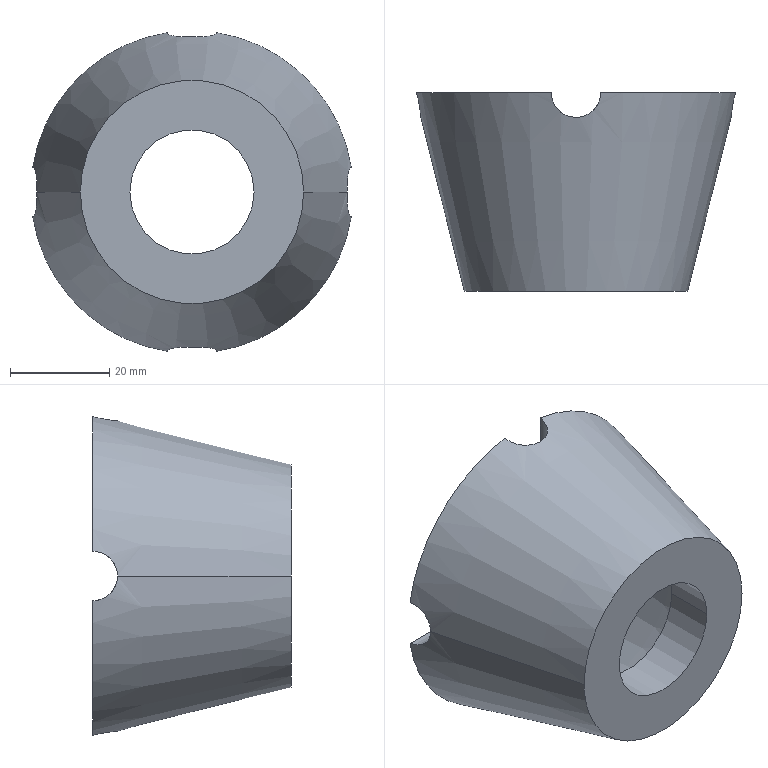Part | SolidWorks | features ICE 2, CirPattern 1, Revolution 1 | 1 solid | 16 faces | box 64.226 x 40 x 64.226 mm | volume 43850 mm3 | cylinder 6 | plane 6 | cone 4 | commonest cylinder face diameters 10 x4 25 x2
STEP:
#1=CARTESIAN_POINT('',(12.5,-20.,0.));
#2=VERTEX_POINT('',#1);
#3=CARTESIAN_POINT('',(-12.5,-20.,0.));
#4=VERTEX_POINT('',#3);
#5=CARTESIAN_POINT('',(0.,-20.,0.));
#6=DIRECTION('',(0.,1.,0.));
#7=DIRECTION('',(-1.,0.,0.));
#8=AXIS2_PLACEMENT_3D('',#5,#6,#7);
#9=CIRCLE('',#8,12.5);
#10=EDGE_CURVE('',#2,#4,#9,.T.);
#11=ORIENTED_EDGE('',*,*,#10,.F.);
#12=CARTESIAN_POINT('',(12.5,-10.,0.));
#13=VERTEX_POINT('',#12);
#14=CARTESIAN_POINT('',(12.5,-20.,0.));
#15=DIRECTION('',(0.,1.,0.));
#16=VECTOR('',#15,1000.);
#17=LINE('',#14,#16);
#18=EDGE_CURVE('',#2,#13,#17,.T.);
#19=ORIENTED_EDGE('',*,*,#18,.T.);
#20=CARTESIAN_POINT('',(-12.5,-10.,0.));
#21=VERTEX_POINT('',#20);
#22=CARTESIAN_POINT('',(0.,-10.,0.));
#23=DIRECTION('',(0.,1.,0.));
#24=DIRECTION('',(-1.,0.,0.));
#25=AXIS2_PLACEMENT_3D('',#22,#23,#24);
#26=CIRCLE('',#25,12.5);
#27=EDGE_CURVE('',#13,#21,#26,.T.);
#28=ORIENTED_EDGE('',*,*,#27,.T.);
#29=CARTESIAN_POINT('',(-12.5,-20.,0.));
#30=DIRECTION('',(0.,1.,0.));
#31=VECTOR('',#30,1000.);
#32=LINE('',#29,#31);
#33=EDGE_CURVE('',#4,#21,#32,.T.);
#34=ORIENTED_EDGE('',*,*,#33,.F.);
#35=EDGE_LOOP('',(#11,#19,#28,#34));
#36=FACE_OUTER_BOUND('',#35,.T.);
#37=CARTESIAN_POINT('',(0.,-20.,0.));
#38=DIRECTION('',(0.,1.,0.));
#39=DIRECTION('',(-1.,0.,0.));
#40=AXIS2_PLACEMENT_3D('',#37,#38,#39);
#41=CYLINDRICAL_SURFACE('',#40,12.5);
#42=ADVANCED_FACE('',(#36),#41,.F.);
#43=CARTESIAN_POINT('',(-22.5,-20.,0.));
#44=VERTEX_POINT('',#43);
#45=CARTESIAN_POINT('',(22.5,-20.,0.));
#46=VERTEX_POINT('',#45);
#47=CARTESIAN_POINT('',(0.,-20.,0.));
#48=DIRECTION('',(0.,1.,0.));
#49=DIRECTION('',(-1.,0.,0.));
#50=AXIS2_PLACEMENT_3D('',#47,#48,#49);
#51=CIRCLE('',#50,22.5);
#52=EDGE_CURVE('',#44,#46,#51,.T.);
#53=ORIENTED_EDGE('',*,*,#52,.T.);
#54=CARTESIAN_POINT('',(31.25,15.,0.));
#55=VERTEX_POINT('',#54);
#56=CARTESIAN_POINT('',(22.5,-20.,0.));
#57=DIRECTION('',(0.2425,0.9701,0.));
#58=VECTOR('',#57,1000.);
#59=LINE('',#56,#58);
#60=EDGE_CURVE('',#46,#55,#59,.T.);
#61=ORIENTED_EDGE('',*,*,#60,.T.);
#62=CARTESIAN_POINT('',(32.113,20.,5.));
#63=VERTEX_POINT('',#62);
#64=CARTESIAN_POINT('',(31.25,15.,0.));
#65=CARTESIAN_POINT('',(31.25,15.,0.3288));
#66=CARTESIAN_POINT('',(31.253,15.033,0.6628));
#67=CARTESIAN_POINT('',(31.265,15.163,1.309));
#68=CARTESIAN_POINT('',(31.274,15.259,1.623));
#69=CARTESIAN_POINT('',(31.294,15.45,2.08));
#70=CARTESIAN_POINT('',(31.301,15.522,2.23));
#71=CARTESIAN_POINT('',(31.319,15.679,2.521));
#72=CARTESIAN_POINT('',(31.328,15.764,2.662));
#73=CARTESIAN_POINT('',(31.361,16.039,3.069));
#74=CARTESIAN_POINT('',(31.388,16.249,3.322));
#75=CARTESIAN_POINT('',(31.453,16.72,3.788));
#76=CARTESIAN_POINT('',(31.492,16.974,3.994));
#77=CARTESIAN_POINT('',(31.581,17.517,4.352));
#78=CARTESIAN_POINT('',(31.633,17.81,4.507));
#79=CARTESIAN_POINT('',(31.749,18.412,4.752));
#80=CARTESIAN_POINT('',(31.813,18.72,4.844));
#81=CARTESIAN_POINT('',(31.954,19.353,4.968));
#82=CARTESIAN_POINT('',(32.031,19.677,5.));
#83=CARTESIAN_POINT('',(32.113,20.,5.));
#84=B_SPLINE_CURVE_WITH_KNOTS('',3,(#64,#65,#66,#67,#68,#69,#70,#71,#72,#73,#74,#75,#76,#77,#78,#79,#80,#81,#82,#83),.UNSPECIFIED.,.F.,.F.,(4,2,2,2,2,2,2,2,2,4),(0.007888,0.008873,0.009858,0.01035,0.01084,0.01183,0.01281,0.0138,0.01478,0.01577),.UNSPECIFIED.);
#85=EDGE_CURVE('',#55,#63,#84,.T.);
#86=ORIENTED_EDGE('',*,*,#85,.T.);
#87=CARTESIAN_POINT('',(5.,20.,32.113));
#88=VERTEX_POINT('',#87);
#89=CARTESIAN_POINT('',(0.,20.,0.));
#90=DIRECTION('',(0.,1.,0.));
#91=DIRECTION('',(-1.,0.,0.));
#92=AXIS2_PLACEMENT_3D('',#89,#90,#91);
#93=CIRCLE('',#92,32.5);
#94=EDGE_CURVE('',#88,#63,#93,.T.);
#95=ORIENTED_EDGE('',*,*,#94,.F.);
#96=CARTESIAN_POINT('',(-5.,20.,32.113));
#97=VERTEX_POINT('',#96);
#98=CARTESIAN_POINT('',(5.,20.,32.113));
#99=CARTESIAN_POINT('',(5.,19.677,32.031));
#100=CARTESIAN_POINT('',(4.969,19.358,31.956));
#101=CARTESIAN_POINT('',(4.877,18.886,31.85));
#102=CARTESIAN_POINT('',(4.838,18.729,31.816));
#103=CARTESIAN_POINT('',(4.746,18.418,31.752));
#104=CARTESIAN_POINT('',(4.691,18.263,31.721));
#105=CARTESIAN_POINT('',(4.507,17.811,31.633));
#106=CARTESIAN_POINT('',(4.356,17.524,31.582));
#107=CARTESIAN_POINT('',(3.997,16.979,31.492));
#108=CARTESIAN_POINT('',(3.787,16.719,31.453));
#109=CARTESIAN_POINT('',(3.327,16.253,31.388));
#110=CARTESIAN_POINT('',(3.075,16.044,31.362));
#111=CARTESIAN_POINT('',(2.665,15.766,31.329));
#112=CARTESIAN_POINT('',(2.522,15.679,31.319));
#113=CARTESIAN_POINT('',(2.231,15.523,31.302));
#114=CARTESIAN_POINT('',(2.083,15.452,31.294));
#115=CARTESIAN_POINT('',(1.629,15.261,31.274));
#116=CARTESIAN_POINT('',(1.312,15.164,31.265));
#117=CARTESIAN_POINT('',(0.6608,15.033,31.253));
#118=CARTESIAN_POINT('',(0.3335,15.,31.25));
#119=CARTESIAN_POINT('',(-0.3245,15.,31.25));
#120=CARTESIAN_POINT('',(-0.6586,15.033,31.253));
#121=CARTESIAN_POINT('',(-1.305,15.162,31.265));
#122=CARTESIAN_POINT('',(-1.619,15.258,31.274));
#123=CARTESIAN_POINT('',(-2.077,15.449,31.294));
#124=CARTESIAN_POINT('',(-2.228,15.521,31.301));
#125=CARTESIAN_POINT('',(-2.519,15.677,31.319));
#126=CARTESIAN_POINT('',(-2.659,15.763,31.328));
#127=CARTESIAN_POINT('',(-3.067,16.038,31.361));
#128=CARTESIAN_POINT('',(-3.32,16.247,31.387));
#129=CARTESIAN_POINT('',(-3.787,16.718,31.453));
#130=CARTESIAN_POINT('',(-3.992,16.972,31.491));
#131=CARTESIAN_POINT('',(-4.351,17.516,31.581));
#132=CARTESIAN_POINT('',(-4.506,17.809,31.633));
#133=CARTESIAN_POINT('',(-4.752,18.411,31.749));
#134=CARTESIAN_POINT('',(-4.844,18.72,31.813));
#135=CARTESIAN_POINT('',(-4.968,19.353,31.954));
#136=CARTESIAN_POINT('',(-5.,19.677,32.031));
#137=CARTESIAN_POINT('',(-5.,20.,32.113));
#138=B_SPLINE_CURVE_WITH_KNOTS('',3,(#98,#99,#100,#101,#102,#103,#104,#105,#106,#107,#108,#109,#110,#111,#112,#113,#114,#115,#116,#117,#118,#119,#120,#121,#122,#123,#124,#125,#126,#127,#128,#129,#130,#131,#132,#133,#134,#135,#136,#137),.UNSPECIFIED.,.F.,.F.,(4,2,2,2,2,2,2,2,2,2,2,2,2,2,2,2,2,2,2,4),(0.000000203,0.0009857,0.001478,0.001971,0.002957,0.003942,0.004927,0.00542,0.005913,0.006898,0.007884,0.008869,0.009855,0.01035,0.01084,0.01183,0.01281,0.0138,0.01478,0.01577),.UNSPECIFIED.);
#139=EDGE_CURVE('',#88,#97,#138,.T.);
#140=ORIENTED_EDGE('',*,*,#139,.T.);
#141=CARTESIAN_POINT('',(-32.113,20.,5.));
#142=VERTEX_POINT('',#141);
#143=CARTESIAN_POINT('',(0.,20.,0.));
#144=DIRECTION('',(0.,1.,0.));
#145=DIRECTION('',(-1.,0.,0.));
#146=AXIS2_PLACEMENT_3D('',#143,#144,#145);
#147=CIRCLE('',#146,32.5);
#148=EDGE_CURVE('',#142,#97,#147,.T.);
#149=ORIENTED_EDGE('',*,*,#148,.F.);
#150=CARTESIAN_POINT('',(-31.25,15.,0.));
#151=VERTEX_POINT('',#150);
#152=CARTESIAN_POINT('',(-32.113,20.,5.));
#153=CARTESIAN_POINT('',(-32.031,19.677,5.));
#154=CARTESIAN_POINT('',(-31.955,19.358,4.969));
#155=CARTESIAN_POINT('',(-31.85,18.885,4.877));
#156=CARTESIAN_POINT('',(-31.816,18.728,4.838));
#157=CARTESIAN_POINT('',(-31.752,18.417,4.746));
#158=CARTESIAN_POINT('',(-31.721,18.262,4.691));
#159=CARTESIAN_POINT('',(-31.633,17.81,4.506));
#160=CARTESIAN_POINT('',(-31.582,17.522,4.355));
#161=CARTESIAN_POINT('',(-31.492,16.977,3.996));
#162=CARTESIAN_POINT('',(-31.453,16.718,3.786));
#163=CARTESIAN_POINT('',(-31.388,16.252,3.325));
#164=CARTESIAN_POINT('',(-31.361,16.042,3.073));
#165=CARTESIAN_POINT('',(-31.328,15.764,2.662));
#166=CARTESIAN_POINT('',(-31.319,15.678,2.519));
#167=CARTESIAN_POINT('',(-31.301,15.521,2.229));
#168=CARTESIAN_POINT('',(-31.294,15.45,2.08));
#169=CARTESIAN_POINT('',(-31.274,15.26,1.626));
#170=CARTESIAN_POINT('',(-31.265,15.163,1.308));
#171=CARTESIAN_POINT('',(-31.253,15.032,0.6567));
#172=CARTESIAN_POINT('',(-31.25,15.,0.3292));
#173=CARTESIAN_POINT('',(-31.25,15.,0.));
#174=B_SPLINE_CURVE_WITH_KNOTS('',3,(#152,#153,#154,#155,#156,#157,#158,#159,#160,#161,#162,#163,#164,#165,#166,#167,#168,#169,#170,#171,#172,#173),.UNSPECIFIED.,.F.,.F.,(4,2,2,2,2,2,2,2,2,2,4),(0.000000203,0.0009862,0.001479,0.001972,0.002958,0.003944,0.00493,0.005423,0.005916,0.006902,0.007888),.UNSPECIFIED.);
#175=EDGE_CURVE('',#142,#151,#174,.T.);
#176=ORIENTED_EDGE('',*,*,#175,.T.);
#177=CARTESIAN_POINT('',(-22.5,-20.,0.));
#178=DIRECTION('',(-0.2425,0.9701,0.));
#179=VECTOR('',#178,1000.);
#180=LINE('',#177,#179);
#181=EDGE_CURVE('',#44,#151,#180,.T.);
#182=ORIENTED_EDGE('',*,*,#181,.F.);
#183=EDGE_LOOP('',(#53,#61,#86,#95,#140,#149,#176,#182));
#184=FACE_OUTER_BOUND('',#183,.T.);
#185=CARTESIAN_POINT('',(0.,-20.,0.));
#186=DIRECTION('',(0.,1.,0.));
#187=DIRECTION('',(-1.,0.,0.));
#188=AXIS2_PLACEMENT_3D('',#185,#186,#187);
#189=CONICAL_SURFACE('',#188,22.5,0.245);
#190=ADVANCED_FACE('',(#184),#189,.T.);
#191=CARTESIAN_POINT('',(18.3,-10.,0.));
#192=VERTEX_POINT('',#191);
#193=CARTESIAN_POINT('',(-18.3,-10.,0.));
#194=VERTEX_POINT('',#193);
#195=CARTESIAN_POINT('',(0.,-10.,0.));
#196=DIRECTION('',(0.,1.,0.));
#197=DIRECTION('',(-1.,0.,0.));
#198=AXIS2_PLACEMENT_3D('',#195,#196,#197);
#199=CIRCLE('',#198,18.3);
#200=EDGE_CURVE('',#192,#194,#199,.T.);
#201=ORIENTED_EDGE('',*,*,#200,.F.);
#202=CARTESIAN_POINT('',(24.55,15.,0.));
#203=VERTEX_POINT('',#202);
#204=CARTESIAN_POINT('',(25.8,20.,0.));
#205=DIRECTION('',(0.2425,0.9701,0.));
#206=VECTOR('',#205,1000.);
#207=LINE('',#204,#206);
#208=EDGE_CURVE('',#192,#203,#207,.T.);
#209=ORIENTED_EDGE('',*,*,#208,.T.);
#210=CARTESIAN_POINT('',(25.311,20.,-5.));
#211=VERTEX_POINT('',#210);
#212=CARTESIAN_POINT('',(24.55,15.,0.));
#213=CARTESIAN_POINT('',(24.55,15.,-0.3286));
#214=CARTESIAN_POINT('',(24.551,15.033,-0.6623));
#215=CARTESIAN_POINT('',(24.558,15.163,-1.307));
#216=CARTESIAN_POINT('',(24.563,15.258,-1.621));
#217=CARTESIAN_POINT('',(24.575,15.449,-2.078));
#218=CARTESIAN_POINT('',(24.58,15.521,-2.229));
#219=CARTESIAN_POINT('',(24.591,15.678,-2.519));
#220=CARTESIAN_POINT('',(24.598,15.763,-2.66));
#221=CARTESIAN_POINT('',(24.621,16.038,-3.067));
#222=CARTESIAN_POINT('',(24.64,16.248,-3.321));
#223=CARTESIAN_POINT('',(24.692,16.718,-3.787));
#224=CARTESIAN_POINT('',(24.723,16.972,-3.992));
#225=CARTESIAN_POINT('',(24.801,17.516,-4.352));
#226=CARTESIAN_POINT('',(24.847,17.81,-4.506));
#227=CARTESIAN_POINT('',(24.955,18.412,-4.752));
#228=CARTESIAN_POINT('',(25.015,18.721,-4.844));
#229=CARTESIAN_POINT('',(25.152,19.354,-4.969));
#230=CARTESIAN_POINT('',(25.229,19.678,-5.));
#231=CARTESIAN_POINT('',(25.311,20.,-5.));
#232=B_SPLINE_CURVE_WITH_KNOTS('',3,(#212,#213,#214,#215,#216,#217,#218,#219,#220,#221,#222,#223,#224,#225,#226,#227,#228,#229,#230,#231),.UNSPECIFIED.,.F.,.F.,(4,2,2,2,2,2,2,2,2,4),(0.007879,0.008863,0.009847,0.01034,0.01083,0.01181,0.0128,0.01378,0.01477,0.01575),.UNSPECIFIED.);
#233=EDGE_CURVE('',#203,#211,#232,.T.);
#234=ORIENTED_EDGE('',*,*,#233,.T.);
#235=CARTESIAN_POINT('',(5.,20.,-25.311));
#236=VERTEX_POINT('',#235);
#237=CARTESIAN_POINT('',(0.,20.,0.));
#238=DIRECTION('',(0.,1.,0.));
#239=DIRECTION('',(-1.,0.,0.));
#240=AXIS2_PLACEMENT_3D('',#237,#238,#239);
#241=CIRCLE('',#240,25.8);
#242=EDGE_CURVE('',#211,#236,#241,.T.);
#243=ORIENTED_EDGE('',*,*,#242,.T.);
#244=CARTESIAN_POINT('',(-5.,20.,-25.311));
#245=VERTEX_POINT('',#244);
#246=CARTESIAN_POINT('',(5.,20.,-25.311));
#247=CARTESIAN_POINT('',(5.,19.678,-25.229));
#248=CARTESIAN_POINT('',(4.969,19.359,-25.154));
#249=CARTESIAN_POINT('',(4.877,18.886,-25.051));
#250=CARTESIAN_POINT('',(4.839,18.73,-25.019));
#251=CARTESIAN_POINT('',(4.746,18.418,-24.957));
#252=CARTESIAN_POINT('',(4.691,18.263,-24.928));
#253=CARTESIAN_POINT('',(4.507,17.81,-24.847));
#254=CARTESIAN_POINT('',(4.356,17.523,-24.802));
#255=CARTESIAN_POINT('',(3.996,16.977,-24.724));
#256=CARTESIAN_POINT('',(3.786,16.718,-24.692));
#257=CARTESIAN_POINT('',(3.325,16.252,-24.641));
#258=CARTESIAN_POINT('',(3.073,16.042,-24.621));
#259=CARTESIAN_POINT('',(2.525,15.672,-24.59));
#260=CARTESIAN_POINT('',(2.232,15.514,-24.579));
#261=CARTESIAN_POINT('',(1.627,15.261,-24.563));
#262=CARTESIAN_POINT('',(1.309,15.163,-24.558));
#263=CARTESIAN_POINT('',(0.6598,15.033,-24.551));
#264=CARTESIAN_POINT('',(0.333,15.,-24.55));
#265=CARTESIAN_POINT('',(-0.3244,15.,-24.55));
#266=CARTESIAN_POINT('',(-0.6583,15.033,-24.551));
#267=CARTESIAN_POINT('',(-1.304,15.162,-24.558));
#268=CARTESIAN_POINT('',(-1.618,15.257,-24.563));
#269=CARTESIAN_POINT('',(-2.075,15.448,-24.575));
#270=CARTESIAN_POINT('',(-2.226,15.52,-24.58));
#271=CARTESIAN_POINT('',(-2.517,15.676,-24.591));
#272=CARTESIAN_POINT('',(-2.657,15.761,-24.598));
#273=CARTESIAN_POINT('',(-3.065,16.036,-24.62));
#274=CARTESIAN_POINT('',(-3.319,16.246,-24.64));
#275=CARTESIAN_POINT('',(-3.785,16.717,-24.692));
#276=CARTESIAN_POINT('',(-3.991,16.971,-24.723));
#277=CARTESIAN_POINT('',(-4.351,17.515,-24.801));
#278=CARTESIAN_POINT('',(-4.506,17.808,-24.847));
#279=CARTESIAN_POINT('',(-4.752,18.411,-24.954));
#280=CARTESIAN_POINT('',(-4.844,18.72,-25.015));
#281=CARTESIAN_POINT('',(-4.968,19.353,-25.152));
#282=CARTESIAN_POINT('',(-5.,19.678,-25.229));
#283=CARTESIAN_POINT('',(-5.,20.,-25.311));
#284=B_SPLINE_CURVE_WITH_KNOTS('',3,(#246,#247,#248,#249,#250,#251,#252,#253,#254,#255,#256,#257,#258,#259,#260,#261,#262,#263,#264,#265,#266,#267,#268,#269,#270,#271,#272,#273,#274,#275,#276,#277,#278,#279,#280,#281,#282,#283),.UNSPECIFIED.,.F.,.F.,(4,2,2,2,2,2,2,2,2,2,2,2,2,2,2,2,2,2,4),(0.000000204,0.0009846,0.001477,0.001969,0.002953,0.003938,0.004922,0.005906,0.006891,0.007875,0.008859,0.009844,0.01034,0.01083,0.01181,0.0128,0.01378,0.01477,0.01575),.UNSPECIFIED.);
#285=EDGE_CURVE('',#236,#245,#284,.T.);
#286=ORIENTED_EDGE('',*,*,#285,.T.);
#287=CARTESIAN_POINT('',(-25.311,20.,-5.));
#288=VERTEX_POINT('',#287);
#289=CARTESIAN_POINT('',(0.,20.,0.));
#290=DIRECTION('',(0.,1.,0.));
#291=DIRECTION('',(-1.,0.,0.));
#292=AXIS2_PLACEMENT_3D('',#289,#290,#291);
#293=CIRCLE('',#292,25.8);
#294=EDGE_CURVE('',#245,#288,#293,.T.);
#295=ORIENTED_EDGE('',*,*,#294,.T.);
#296=CARTESIAN_POINT('',(-24.55,15.,0.));
#297=VERTEX_POINT('',#296);
#298=CARTESIAN_POINT('',(-25.311,20.,-5.));
#299=CARTESIAN_POINT('',(-25.229,19.677,-5.));
#300=CARTESIAN_POINT('',(-25.154,19.359,-4.969));
#301=CARTESIAN_POINT('',(-25.051,18.886,-4.877));
#302=CARTESIAN_POINT('',(-25.019,18.729,-4.838));
#303=CARTESIAN_POINT('',(-24.957,18.417,-4.746));
#304=CARTESIAN_POINT('',(-24.928,18.262,-4.691));
#305=CARTESIAN_POINT('',(-24.847,17.809,-4.506));
#306=CARTESIAN_POINT('',(-24.802,17.522,-4.355));
#307=CARTESIAN_POINT('',(-24.724,16.976,-3.995));
#308=CARTESIAN_POINT('',(-24.692,16.716,-3.785));
#309=CARTESIAN_POINT('',(-24.64,16.25,-3.324));
#310=CARTESIAN_POINT('',(-24.621,16.041,-3.071));
#311=CARTESIAN_POINT('',(-24.59,15.67,-2.522));
#312=CARTESIAN_POINT('',(-24.579,15.513,-2.23));
#313=CARTESIAN_POINT('',(-24.563,15.26,-1.624));
#314=CARTESIAN_POINT('',(-24.558,15.162,-1.306));
#315=CARTESIAN_POINT('',(-24.551,15.032,-0.6559));
#316=CARTESIAN_POINT('',(-24.55,15.,-0.3289));
#317=CARTESIAN_POINT('',(-24.55,15.,0.));
#318=B_SPLINE_CURVE_WITH_KNOTS('',3,(#298,#299,#300,#301,#302,#303,#304,#305,#306,#307,#308,#309,#310,#311,#312,#313,#314,#315,#316,#317),.UNSPECIFIED.,.F.,.F.,(4,2,2,2,2,2,2,2,2,4),(0.000000204,0.0009851,0.001478,0.00197,0.002955,0.00394,0.004925,0.00591,0.006894,0.007879),.UNSPECIFIED.);
#319=EDGE_CURVE('',#288,#297,#318,.T.);
#320=ORIENTED_EDGE('',*,*,#319,.T.);
#321=CARTESIAN_POINT('',(-25.8,20.,0.));
#322=DIRECTION('',(-0.2425,0.9701,0.));
#323=VECTOR('',#322,1000.);
#324=LINE('',#321,#323);
#325=EDGE_CURVE('',#194,#297,#324,.T.);
#326=ORIENTED_EDGE('',*,*,#325,.F.);
#327=EDGE_LOOP('',(#201,#209,#234,#243,#286,#295,#320,#326));
#328=FACE_OUTER_BOUND('',#327,.T.);
#329=CARTESIAN_POINT('',(0.,20.,0.));
#330=DIRECTION('',(0.,1.,0.));
#331=DIRECTION('',(-1.,0.,0.));
#332=AXIS2_PLACEMENT_3D('',#329,#330,#331);
#333=CONICAL_SURFACE('',#332,25.8,0.245);
#334=ADVANCED_FACE('',(#328),#333,.F.);
#335=ORIENTED_EDGE('',*,*,#94,.T.);
#336=CARTESIAN_POINT('',(25.311,20.,5.));
#337=VERTEX_POINT('',#336);
#338=CARTESIAN_POINT('',(40.,20.,5.));
#339=DIRECTION('',(-1.,0.,0.));
#340=VECTOR('',#339,1000.);
#341=LINE('',#338,#340);
#342=EDGE_CURVE('',#63,#337,#341,.T.);
#343=ORIENTED_EDGE('',*,*,#342,.T.);
#344=CARTESIAN_POINT('',(5.,20.,25.311));
#345=VERTEX_POINT('',#344);
#346=CARTESIAN_POINT('',(0.,20.,0.));
#347=DIRECTION('',(0.,1.,0.));
#348=DIRECTION('',(-1.,0.,0.));
#349=AXIS2_PLACEMENT_3D('',#346,#347,#348);
#350=CIRCLE('',#349,25.8);
#351=EDGE_CURVE('',#345,#337,#350,.T.);
#352=ORIENTED_EDGE('',*,*,#351,.F.);
#353=CARTESIAN_POINT('',(5.,20.,-40.));
#354=DIRECTION('',(0.,0.,1.));
#355=VECTOR('',#354,1000.);
#356=LINE('',#353,#355);
#357=EDGE_CURVE('',#345,#88,#356,.T.);
#358=ORIENTED_EDGE('',*,*,#357,.T.);
#359=EDGE_LOOP('',(#335,#343,#352,#358));
#360=FACE_OUTER_BOUND('',#359,.T.);
#361=CARTESIAN_POINT('',(32.5,20.,0.));
#362=DIRECTION('',(0.,-1.,0.));
#363=DIRECTION('',(1.,0.,0.));
#364=AXIS2_PLACEMENT_3D('',#361,#362,#363);
#365=PLANE('',#364);
#366=ADVANCED_FACE('',(#360),#365,.F.);
#367=CARTESIAN_POINT('',(-25.311,20.,5.));
#368=VERTEX_POINT('',#367);
#369=CARTESIAN_POINT('',(-5.,20.,25.311));
#370=VERTEX_POINT('',#369);
#371=CARTESIAN_POINT('',(0.,20.,0.));
#372=DIRECTION('',(0.,1.,0.));
#373=DIRECTION('',(-1.,0.,0.));
#374=AXIS2_PLACEMENT_3D('',#371,#372,#373);
#375=CIRCLE('',#374,25.8);
#376=EDGE_CURVE('',#368,#370,#375,.T.);
#377=ORIENTED_EDGE('',*,*,#376,.F.);
#378=CARTESIAN_POINT('',(40.,20.,5.));
#379=DIRECTION('',(-1.,0.,0.));
#380=VECTOR('',#379,1000.);
#381=LINE('',#378,#380);
#382=EDGE_CURVE('',#368,#142,#381,.T.);
#383=ORIENTED_EDGE('',*,*,#382,.T.);
#384=ORIENTED_EDGE('',*,*,#148,.T.);
#385=CARTESIAN_POINT('',(-5.,20.,-40.));
#386=DIRECTION('',(0.,0.,1.));
#387=VECTOR('',#386,1000.);
#388=LINE('',#385,#387);
#389=EDGE_CURVE('',#370,#97,#388,.T.);
#390=ORIENTED_EDGE('',*,*,#389,.F.);
#391=EDGE_LOOP('',(#377,#383,#384,#390));
#392=FACE_OUTER_BOUND('',#391,.T.);
#393=CARTESIAN_POINT('',(32.5,20.,0.));
#394=DIRECTION('',(0.,-1.,0.));
#395=DIRECTION('',(1.,0.,0.));
#396=AXIS2_PLACEMENT_3D('',#393,#394,#395);
#397=PLANE('',#396);
#398=ADVANCED_FACE('',(#392),#397,.F.);
#399=ORIENTED_EDGE('',*,*,#242,.F.);
#400=CARTESIAN_POINT('',(32.113,20.,-5.));
#401=VERTEX_POINT('',#400);
#402=CARTESIAN_POINT('',(40.,20.,-5.));
#403=DIRECTION('',(-1.,0.,0.));
#404=VECTOR('',#403,1000.);
#405=LINE('',#402,#404);
#406=EDGE_CURVE('',#401,#211,#405,.T.);
#407=ORIENTED_EDGE('',*,*,#406,.F.);
#408=CARTESIAN_POINT('',(5.,20.,-32.113));
#409=VERTEX_POINT('',#408);
#410=CARTESIAN_POINT('',(0.,20.,0.));
#411=DIRECTION('',(0.,1.,0.));
#412=DIRECTION('',(-1.,0.,0.));
#413=AXIS2_PLACEMENT_3D('',#410,#411,#412);
#414=CIRCLE('',#413,32.5);
#415=EDGE_CURVE('',#401,#409,#414,.T.);
#416=ORIENTED_EDGE('',*,*,#415,.T.);
#417=CARTESIAN_POINT('',(5.,20.,-40.));
#418=DIRECTION('',(0.,0.,1.));
#419=VECTOR('',#418,1000.);
#420=LINE('',#417,#419);
#421=EDGE_CURVE('',#409,#236,#420,.T.);
#422=ORIENTED_EDGE('',*,*,#421,.T.);
#423=EDGE_LOOP('',(#399,#407,#416,#422));
#424=FACE_OUTER_BOUND('',#423,.T.);
#425=CARTESIAN_POINT('',(32.5,20.,0.));
#426=DIRECTION('',(0.,-1.,0.));
#427=DIRECTION('',(1.,0.,0.));
#428=AXIS2_PLACEMENT_3D('',#425,#426,#427);
#429=PLANE('',#428);
#430=ADVANCED_FACE('',(#424),#429,.F.);
#431=CARTESIAN_POINT('',(0.,-10.,0.));
#432=DIRECTION('',(0.,1.,0.));
#433=DIRECTION('',(-1.,0.,0.));
#434=AXIS2_PLACEMENT_3D('',#431,#432,#433);
#435=CIRCLE('',#434,12.5);
#436=EDGE_CURVE('',#21,#13,#435,.T.);
#437=ORIENTED_EDGE('',*,*,#436,.F.);
#438=ORIENTED_EDGE('',*,*,#27,.F.);
#439=EDGE_LOOP('',(#437,#438));
#440=FACE_BOUND('',#439,.T.);
#441=CARTESIAN_POINT('',(0.,-10.,0.));
#442=DIRECTION('',(0.,1.,0.));
#443=DIRECTION('',(-1.,0.,0.));
#444=AXIS2_PLACEMENT_3D('',#441,#442,#443);
#445=CIRCLE('',#444,18.3);
#446=EDGE_CURVE('',#194,#192,#445,.T.);
#447=ORIENTED_EDGE('',*,*,#446,.T.);
#448=ORIENTED_EDGE('',*,*,#200,.T.);
#449=EDGE_LOOP('',(#447,#448));
#450=FACE_OUTER_BOUND('',#449,.T.);
#451=CARTESIAN_POINT('',(0.,-10.,0.));
#452=DIRECTION('',(0.,-1.,0.));
#453=DIRECTION('',(1.,0.,0.));
#454=AXIS2_PLACEMENT_3D('',#451,#452,#453);
#455=PLANE('',#454);
#456=ADVANCED_FACE('',(#440,#450),#455,.F.);
#457=ORIENTED_EDGE('',*,*,#208,.F.);
#458=ORIENTED_EDGE('',*,*,#446,.F.);
#459=ORIENTED_EDGE('',*,*,#325,.T.);
#460=CARTESIAN_POINT('',(-24.55,15.,0.));
#461=CARTESIAN_POINT('',(-24.55,15.,0.3286));
#462=CARTESIAN_POINT('',(-24.551,15.033,0.6623));
#463=CARTESIAN_POINT('',(-24.558,15.163,1.307));
#464=CARTESIAN_POINT('',(-24.563,15.258,1.621));
#465=CARTESIAN_POINT('',(-24.575,15.449,2.078));
#466=CARTESIAN_POINT('',(-24.58,15.521,2.229));
#467=CARTESIAN_POINT('',(-24.591,15.678,2.519));
#468=CARTESIAN_POINT('',(-24.598,15.763,2.66));
#469=CARTESIAN_POINT('',(-24.621,16.038,3.067));
#470=CARTESIAN_POINT('',(-24.64,16.248,3.321));
#471=CARTESIAN_POINT('',(-24.692,16.718,3.787));
#472=CARTESIAN_POINT('',(-24.723,16.972,3.992));
#473=CARTESIAN_POINT('',(-24.801,17.516,4.352));
#474=CARTESIAN_POINT('',(-24.847,17.81,4.506));
#475=CARTESIAN_POINT('',(-24.955,18.412,4.752));
#476=CARTESIAN_POINT('',(-25.015,18.721,4.844));
#477=CARTESIAN_POINT('',(-25.152,19.354,4.969));
#478=CARTESIAN_POINT('',(-25.229,19.678,5.));
#479=CARTESIAN_POINT('',(-25.311,20.,5.));
#480=B_SPLINE_CURVE_WITH_KNOTS('',3,(#460,#461,#462,#463,#464,#465,#466,#467,#468,#469,#470,#471,#472,#473,#474,#475,#476,#477,#478,#479),.UNSPECIFIED.,.F.,.F.,(4,2,2,2,2,2,2,2,2,4),(0.007879,0.008863,0.009847,0.01034,0.01083,0.01181,0.0128,0.01378,0.01477,0.01575),.UNSPECIFIED.);
#481=EDGE_CURVE('',#297,#368,#480,.T.);
#482=ORIENTED_EDGE('',*,*,#481,.T.);
#483=ORIENTED_EDGE('',*,*,#376,.T.);
#484=CARTESIAN_POINT('',(-5.,20.,25.311));
#485=CARTESIAN_POINT('',(-5.,19.678,25.229));
#486=CARTESIAN_POINT('',(-4.969,19.359,25.154));
#487=CARTESIAN_POINT('',(-4.877,18.886,25.051));
#488=CARTESIAN_POINT('',(-4.839,18.73,25.019));
#489=CARTESIAN_POINT('',(-4.746,18.418,24.957));
#490=CARTESIAN_POINT('',(-4.691,18.263,24.928));
#491=CARTESIAN_POINT('',(-4.507,17.81,24.847));
#492=CARTESIAN_POINT('',(-4.356,17.523,24.802));
#493=CARTESIAN_POINT('',(-3.996,16.977,24.724));
#494=CARTESIAN_POINT('',(-3.786,16.718,24.692));
#495=CARTESIAN_POINT('',(-3.325,16.252,24.641));
#496=CARTESIAN_POINT('',(-3.073,16.042,24.621));
#497=CARTESIAN_POINT('',(-2.525,15.672,24.59));
#498=CARTESIAN_POINT('',(-2.232,15.514,24.579));
#499=CARTESIAN_POINT('',(-1.627,15.261,24.563));
#500=CARTESIAN_POINT('',(-1.309,15.163,24.558));
#501=CARTESIAN_POINT('',(-0.6598,15.033,24.551));
#502=CARTESIAN_POINT('',(-0.333,15.,24.55));
#503=CARTESIAN_POINT('',(0.3244,15.,24.55));
#504=CARTESIAN_POINT('',(0.6583,15.033,24.551));
#505=CARTESIAN_POINT('',(1.304,15.162,24.558));
#506=CARTESIAN_POINT('',(1.618,15.257,24.563));
#507=CARTESIAN_POINT('',(2.075,15.448,24.575));
#508=CARTESIAN_POINT('',(2.226,15.52,24.58));
#509=CARTESIAN_POINT('',(2.517,15.676,24.591));
#510=CARTESIAN_POINT('',(2.657,15.761,24.598));
#511=CARTESIAN_POINT('',(3.065,16.036,24.62));
#512=CARTESIAN_POINT('',(3.319,16.246,24.64));
#513=CARTESIAN_POINT('',(3.785,16.717,24.692));
#514=CARTESIAN_POINT('',(3.991,16.971,24.723));
#515=CARTESIAN_POINT('',(4.351,17.515,24.801));
#516=CARTESIAN_POINT('',(4.506,17.808,24.847));
#517=CARTESIAN_POINT('',(4.752,18.411,24.954));
#518=CARTESIAN_POINT('',(4.844,18.72,25.015));
#519=CARTESIAN_POINT('',(4.968,19.353,25.152));
#520=CARTESIAN_POINT('',(5.,19.678,25.229));
#521=CARTESIAN_POINT('',(5.,20.,25.311));
#522=B_SPLINE_CURVE_WITH_KNOTS('',3,(#484,#485,#486,#487,#488,#489,#490,#491,#492,#493,#494,#495,#496,#497,#498,#499,#500,#501,#502,#503,#504,#505,#506,#507,#508,#509,#510,#511,#512,#513,#514,#515,#516,#517,#518,#519,#520,#521),.UNSPECIFIED.,.F.,.F.,(4,2,2,2,2,2,2,2,2,2,2,2,2,2,2,2,2,2,4),(0.000000204,0.0009846,0.001477,0.001969,0.002953,0.003938,0.004922,0.005906,0.006891,0.007875,0.008859,0.009844,0.01034,0.01083,0.01181,0.0128,0.01378,0.01477,0.01575),.UNSPECIFIED.);
#523=EDGE_CURVE('',#370,#345,#522,.T.);
#524=ORIENTED_EDGE('',*,*,#523,.T.);
#525=ORIENTED_EDGE('',*,*,#351,.T.);
#526=CARTESIAN_POINT('',(25.311,20.,5.));
#527=CARTESIAN_POINT('',(25.229,19.677,5.));
#528=CARTESIAN_POINT('',(25.154,19.359,4.969));
#529=CARTESIAN_POINT('',(25.051,18.886,4.877));
#530=CARTESIAN_POINT('',(25.019,18.729,4.838));
#531=CARTESIAN_POINT('',(24.957,18.417,4.746));
#532=CARTESIAN_POINT('',(24.928,18.262,4.691));
#533=CARTESIAN_POINT('',(24.847,17.809,4.506));
#534=CARTESIAN_POINT('',(24.802,17.522,4.355));
#535=CARTESIAN_POINT('',(24.724,16.976,3.995));
#536=CARTESIAN_POINT('',(24.692,16.716,3.785));
#537=CARTESIAN_POINT('',(24.64,16.25,3.324));
#538=CARTESIAN_POINT('',(24.621,16.041,3.071));
#539=CARTESIAN_POINT('',(24.59,15.67,2.522));
#540=CARTESIAN_POINT('',(24.579,15.513,2.23));
#541=CARTESIAN_POINT('',(24.563,15.26,1.624));
#542=CARTESIAN_POINT('',(24.558,15.162,1.306));
#543=CARTESIAN_POINT('',(24.551,15.032,0.6559));
#544=CARTESIAN_POINT('',(24.55,15.,0.3289));
#545=CARTESIAN_POINT('',(24.55,15.,0.));
#546=B_SPLINE_CURVE_WITH_KNOTS('',3,(#526,#527,#528,#529,#530,#531,#532,#533,#534,#535,#536,#537,#538,#539,#540,#541,#542,#543,#544,#545),.UNSPECIFIED.,.F.,.F.,(4,2,2,2,2,2,2,2,2,4),(0.000000204,0.0009851,0.001478,0.00197,0.002955,0.00394,0.004925,0.00591,0.006894,0.007879),.UNSPECIFIED.);
#547=EDGE_CURVE('',#337,#203,#546,.T.);
#548=ORIENTED_EDGE('',*,*,#547,.T.);
#549=EDGE_LOOP('',(#457,#458,#459,#482,#483,#524,#525,#548));
#550=FACE_OUTER_BOUND('',#549,.T.);
#551=CARTESIAN_POINT('',(0.,20.,0.));
#552=DIRECTION('',(0.,1.,0.));
#553=DIRECTION('',(-1.,0.,0.));
#554=AXIS2_PLACEMENT_3D('',#551,#552,#553);
#555=CONICAL_SURFACE('',#554,25.8,0.245);
#556=ADVANCED_FACE('',(#550),#555,.F.);
#557=CARTESIAN_POINT('',(-5.,20.,-32.113));
#558=VERTEX_POINT('',#557);
#559=CARTESIAN_POINT('',(-32.113,20.,-5.));
#560=VERTEX_POINT('',#559);
#561=CARTESIAN_POINT('',(0.,20.,0.));
#562=DIRECTION('',(0.,1.,0.));
#563=DIRECTION('',(-1.,0.,0.));
#564=AXIS2_PLACEMENT_3D('',#561,#562,#563);
#565=CIRCLE('',#564,32.5);
#566=EDGE_CURVE('',#558,#560,#565,.T.);
#567=ORIENTED_EDGE('',*,*,#566,.T.);
#568=CARTESIAN_POINT('',(40.,20.,-5.));
#569=DIRECTION('',(-1.,0.,0.));
#570=VECTOR('',#569,1000.);
#571=LINE('',#568,#570);
#572=EDGE_CURVE('',#288,#560,#571,.T.);
#573=ORIENTED_EDGE('',*,*,#572,.F.);
#574=ORIENTED_EDGE('',*,*,#294,.F.);
#575=CARTESIAN_POINT('',(-5.,20.,-40.));
#576=DIRECTION('',(0.,0.,1.));
#577=VECTOR('',#576,1000.);
#578=LINE('',#575,#577);
#579=EDGE_CURVE('',#558,#245,#578,.T.);
#580=ORIENTED_EDGE('',*,*,#579,.F.);
#581=EDGE_LOOP('',(#567,#573,#574,#580));
#582=FACE_OUTER_BOUND('',#581,.T.);
#583=CARTESIAN_POINT('',(32.5,20.,0.));
#584=DIRECTION('',(0.,-1.,0.));
#585=DIRECTION('',(1.,0.,0.));
#586=AXIS2_PLACEMENT_3D('',#583,#584,#585);
#587=PLANE('',#586);
#588=ADVANCED_FACE('',(#582),#587,.F.);
#589=ORIENTED_EDGE('',*,*,#60,.F.);
#590=CARTESIAN_POINT('',(0.,-20.,0.));
#591=DIRECTION('',(0.,1.,0.));
#592=DIRECTION('',(-1.,0.,0.));
#593=AXIS2_PLACEMENT_3D('',#590,#591,#592);
#594=CIRCLE('',#593,22.5);
#595=EDGE_CURVE('',#46,#44,#594,.T.);
#596=ORIENTED_EDGE('',*,*,#595,.T.);
#597=ORIENTED_EDGE('',*,*,#181,.T.);
#598=CARTESIAN_POINT('',(-31.25,15.,0.));
#599=CARTESIAN_POINT('',(-31.25,15.,-0.3288));
#600=CARTESIAN_POINT('',(-31.253,15.033,-0.6628));
#601=CARTESIAN_POINT('',(-31.265,15.163,-1.309));
#602=CARTESIAN_POINT('',(-31.274,15.259,-1.623));
#603=CARTESIAN_POINT('',(-31.294,15.45,-2.08));
#604=CARTESIAN_POINT('',(-31.301,15.522,-2.23));
#605=CARTESIAN_POINT('',(-31.319,15.679,-2.521));
#606=CARTESIAN_POINT('',(-31.328,15.764,-2.662));
#607=CARTESIAN_POINT('',(-31.361,16.039,-3.069));
#608=CARTESIAN_POINT('',(-31.388,16.249,-3.322));
#609=CARTESIAN_POINT('',(-31.453,16.72,-3.788));
#610=CARTESIAN_POINT('',(-31.492,16.974,-3.994));
#611=CARTESIAN_POINT('',(-31.581,17.517,-4.352));
#612=CARTESIAN_POINT('',(-31.633,17.81,-4.507));
#613=CARTESIAN_POINT('',(-31.749,18.412,-4.752));
#614=CARTESIAN_POINT('',(-31.813,18.72,-4.844));
#615=CARTESIAN_POINT('',(-31.954,19.353,-4.968));
#616=CARTESIAN_POINT('',(-32.031,19.677,-5.));
#617=CARTESIAN_POINT('',(-32.113,20.,-5.));
#618=B_SPLINE_CURVE_WITH_KNOTS('',3,(#598,#599,#600,#601,#602,#603,#604,#605,#606,#607,#608,#609,#610,#611,#612,#613,#614,#615,#616,#617),.UNSPECIFIED.,.F.,.F.,(4,2,2,2,2,2,2,2,2,4),(0.007888,0.008873,0.009858,0.01035,0.01084,0.01183,0.01281,0.0138,0.01478,0.01577),.UNSPECIFIED.);
#619=EDGE_CURVE('',#151,#560,#618,.T.);
#620=ORIENTED_EDGE('',*,*,#619,.T.);
#621=ORIENTED_EDGE('',*,*,#566,.F.);
#622=CARTESIAN_POINT('',(-5.,20.,-32.113));
#623=CARTESIAN_POINT('',(-5.,19.677,-32.031));
#624=CARTESIAN_POINT('',(-4.969,19.358,-31.956));
#625=CARTESIAN_POINT('',(-4.877,18.886,-31.85));
#626=CARTESIAN_POINT('',(-4.838,18.729,-31.816));
#627=CARTESIAN_POINT('',(-4.746,18.418,-31.752));
#628=CARTESIAN_POINT('',(-4.691,18.263,-31.721));
#629=CARTESIAN_POINT('',(-4.507,17.811,-31.633));
#630=CARTESIAN_POINT('',(-4.356,17.524,-31.582));
#631=CARTESIAN_POINT('',(-3.997,16.979,-31.492));
#632=CARTESIAN_POINT('',(-3.787,16.719,-31.453));
#633=CARTESIAN_POINT('',(-3.327,16.253,-31.388));
#634=CARTESIAN_POINT('',(-3.075,16.044,-31.362));
#635=CARTESIAN_POINT('',(-2.665,15.766,-31.329));
#636=CARTESIAN_POINT('',(-2.522,15.679,-31.319));
#637=CARTESIAN_POINT('',(-2.231,15.523,-31.302));
#638=CARTESIAN_POINT('',(-2.083,15.452,-31.294));
#639=CARTESIAN_POINT('',(-1.629,15.261,-31.274));
#640=CARTESIAN_POINT('',(-1.312,15.164,-31.265));
#641=CARTESIAN_POINT('',(-0.6608,15.033,-31.253));
#642=CARTESIAN_POINT('',(-0.3335,15.,-31.25));
#643=CARTESIAN_POINT('',(0.3245,15.,-31.25));
#644=CARTESIAN_POINT('',(0.6586,15.033,-31.253));
#645=CARTESIAN_POINT('',(1.305,15.162,-31.265));
#646=CARTESIAN_POINT('',(1.619,15.258,-31.274));
#647=CARTESIAN_POINT('',(2.077,15.449,-31.294));
#648=CARTESIAN_POINT('',(2.228,15.521,-31.301));
#649=CARTESIAN_POINT('',(2.519,15.677,-31.319));
#650=CARTESIAN_POINT('',(2.659,15.763,-31.328));
#651=CARTESIAN_POINT('',(3.067,16.038,-31.361));
#652=CARTESIAN_POINT('',(3.32,16.247,-31.387));
#653=CARTESIAN_POINT('',(3.787,16.718,-31.453));
#654=CARTESIAN_POINT('',(3.992,16.972,-31.491));
#655=CARTESIAN_POINT('',(4.351,17.516,-31.581));
#656=CARTESIAN_POINT('',(4.506,17.809,-31.633));
#657=CARTESIAN_POINT('',(4.752,18.411,-31.749));
#658=CARTESIAN_POINT('',(4.844,18.72,-31.813));
#659=CARTESIAN_POINT('',(4.968,19.353,-31.954));
#660=CARTESIAN_POINT('',(5.,19.677,-32.031));
#661=CARTESIAN_POINT('',(5.,20.,-32.113));
#662=B_SPLINE_CURVE_WITH_KNOTS('',3,(#622,#623,#624,#625,#626,#627,#628,#629,#630,#631,#632,#633,#634,#635,#636,#637,#638,#639,#640,#641,#642,#643,#644,#645,#646,#647,#648,#649,#650,#651,#652,#653,#654,#655,#656,#657,#658,#659,#660,#661),.UNSPECIFIED.,.F.,.F.,(4,2,2,2,2,2,2,2,2,2,2,2,2,2,2,2,2,2,2,4),(0.000000203,0.0009857,0.001478,0.001971,0.002957,0.003942,0.004927,0.00542,0.005913,0.006898,0.007884,0.008869,0.009855,0.01035,0.01084,0.01183,0.01281,0.0138,0.01478,0.01577),.UNSPECIFIED.);
#663=EDGE_CURVE('',#558,#409,#662,.T.);
#664=ORIENTED_EDGE('',*,*,#663,.T.);
#665=ORIENTED_EDGE('',*,*,#415,.F.);
#666=CARTESIAN_POINT('',(32.113,20.,-5.));
#667=CARTESIAN_POINT('',(32.031,19.677,-5.));
#668=CARTESIAN_POINT('',(31.955,19.358,-4.969));
#669=CARTESIAN_POINT('',(31.85,18.885,-4.877));
#670=CARTESIAN_POINT('',(31.816,18.728,-4.838));
#671=CARTESIAN_POINT('',(31.752,18.417,-4.746));
#672=CARTESIAN_POINT('',(31.721,18.262,-4.691));
#673=CARTESIAN_POINT('',(31.633,17.81,-4.506));
#674=CARTESIAN_POINT('',(31.582,17.522,-4.355));
#675=CARTESIAN_POINT('',(31.492,16.977,-3.996));
#676=CARTESIAN_POINT('',(31.453,16.718,-3.786));
#677=CARTESIAN_POINT('',(31.388,16.252,-3.325));
#678=CARTESIAN_POINT('',(31.361,16.042,-3.073));
#679=CARTESIAN_POINT('',(31.328,15.764,-2.662));
#680=CARTESIAN_POINT('',(31.319,15.678,-2.519));
#681=CARTESIAN_POINT('',(31.301,15.521,-2.229));
#682=CARTESIAN_POINT('',(31.294,15.45,-2.08));
#683=CARTESIAN_POINT('',(31.274,15.26,-1.626));
#684=CARTESIAN_POINT('',(31.265,15.163,-1.308));
#685=CARTESIAN_POINT('',(31.253,15.032,-0.6567));
#686=CARTESIAN_POINT('',(31.25,15.,-0.3292));
#687=CARTESIAN_POINT('',(31.25,15.,0.));
#688=B_SPLINE_CURVE_WITH_KNOTS('',3,(#666,#667,#668,#669,#670,#671,#672,#673,#674,#675,#676,#677,#678,#679,#680,#681,#682,#683,#684,#685,#686,#687),.UNSPECIFIED.,.F.,.F.,(4,2,2,2,2,2,2,2,2,2,4),(0.000000203,0.0009862,0.001479,0.001972,0.002958,0.003944,0.00493,0.005423,0.005916,0.006902,0.007888),.UNSPECIFIED.);
#689=EDGE_CURVE('',#401,#55,#688,.T.);
#690=ORIENTED_EDGE('',*,*,#689,.T.);
#691=EDGE_LOOP('',(#589,#596,#597,#620,#621,#664,#665,#690));
#692=FACE_OUTER_BOUND('',#691,.T.);
#693=CARTESIAN_POINT('',(0.,-20.,0.));
#694=DIRECTION('',(0.,1.,0.));
#695=DIRECTION('',(-1.,0.,0.));
#696=AXIS2_PLACEMENT_3D('',#693,#694,#695);
#697=CONICAL_SURFACE('',#696,22.5,0.245);
#698=ADVANCED_FACE('',(#692),#697,.T.);
#699=CARTESIAN_POINT('',(0.,-20.,0.));
#700=DIRECTION('',(0.,1.,0.));
#701=DIRECTION('',(-1.,0.,0.));
#702=AXIS2_PLACEMENT_3D('',#699,#700,#701);
#703=CIRCLE('',#702,12.5);
#704=EDGE_CURVE('',#4,#2,#703,.T.);
#705=ORIENTED_EDGE('',*,*,#704,.T.);
#706=ORIENTED_EDGE('',*,*,#10,.T.);
#707=EDGE_LOOP('',(#705,#706));
#708=FACE_BOUND('',#707,.T.);
#709=ORIENTED_EDGE('',*,*,#52,.F.);
#710=ORIENTED_EDGE('',*,*,#595,.F.);
#711=EDGE_LOOP('',(#709,#710));
#712=FACE_OUTER_BOUND('',#711,.T.);
#713=CARTESIAN_POINT('',(22.5,-20.,0.));
#714=DIRECTION('',(0.,1.,0.));
#715=DIRECTION('',(-1.,0.,0.));
#716=AXIS2_PLACEMENT_3D('',#713,#714,#715);
#717=PLANE('',#716);
#718=ADVANCED_FACE('',(#708,#712),#717,.F.);
#719=ORIENTED_EDGE('',*,*,#18,.F.);
#720=ORIENTED_EDGE('',*,*,#704,.F.);
#721=ORIENTED_EDGE('',*,*,#33,.T.);
#722=ORIENTED_EDGE('',*,*,#436,.T.);
#723=EDGE_LOOP('',(#719,#720,#721,#722));
#724=FACE_OUTER_BOUND('',#723,.T.);
#725=CARTESIAN_POINT('',(0.,-20.,0.));
#726=DIRECTION('',(0.,1.,0.));
#727=DIRECTION('',(-1.,0.,0.));
#728=AXIS2_PLACEMENT_3D('',#725,#726,#727);
#729=CYLINDRICAL_SURFACE('',#728,12.5);
#730=ADVANCED_FACE('',(#724),#729,.F.);
#731=ORIENTED_EDGE('',*,*,#421,.F.);
#732=ORIENTED_EDGE('',*,*,#663,.F.);
#733=ORIENTED_EDGE('',*,*,#579,.T.);
#734=ORIENTED_EDGE('',*,*,#285,.F.);
#735=EDGE_LOOP('',(#731,#732,#733,#734));
#736=FACE_OUTER_BOUND('',#735,.T.);
#737=CARTESIAN_POINT('',(0.,20.,-40.));
#738=DIRECTION('',(0.,0.,1.));
#739=DIRECTION('',(1.,0.,0.));
#740=AXIS2_PLACEMENT_3D('',#737,#738,#739);
#741=CYLINDRICAL_SURFACE('',#740,5.);
#742=ADVANCED_FACE('',(#736),#741,.F.);
#743=ORIENTED_EDGE('',*,*,#389,.T.);
#744=ORIENTED_EDGE('',*,*,#139,.F.);
#745=ORIENTED_EDGE('',*,*,#357,.F.);
#746=ORIENTED_EDGE('',*,*,#523,.F.);
#747=EDGE_LOOP('',(#743,#744,#745,#746));
#748=FACE_OUTER_BOUND('',#747,.T.);
#749=CARTESIAN_POINT('',(0.,20.,-40.));
#750=DIRECTION('',(0.,0.,1.));
#751=DIRECTION('',(1.,0.,0.));
#752=AXIS2_PLACEMENT_3D('',#749,#750,#751);
#753=CYLINDRICAL_SURFACE('',#752,5.);
#754=ADVANCED_FACE('',(#748),#753,.F.);
#755=ORIENTED_EDGE('',*,*,#572,.T.);
#756=ORIENTED_EDGE('',*,*,#619,.F.);
#757=ORIENTED_EDGE('',*,*,#175,.F.);
#758=ORIENTED_EDGE('',*,*,#382,.F.);
#759=ORIENTED_EDGE('',*,*,#481,.F.);
#760=ORIENTED_EDGE('',*,*,#319,.F.);
#761=EDGE_LOOP('',(#755,#756,#757,#758,#759,#760));
#762=FACE_OUTER_BOUND('',#761,.T.);
#763=CARTESIAN_POINT('',(40.,20.,0.));
#764=DIRECTION('',(-1.,0.,0.));
#765=DIRECTION('',(0.,0.,1.));
#766=AXIS2_PLACEMENT_3D('',#763,#764,#765);
#767=CYLINDRICAL_SURFACE('',#766,5.);
#768=ADVANCED_FACE('',(#762),#767,.F.);
#769=ORIENTED_EDGE('',*,*,#342,.F.);
#770=ORIENTED_EDGE('',*,*,#85,.F.);
#771=ORIENTED_EDGE('',*,*,#689,.F.);
#772=ORIENTED_EDGE('',*,*,#406,.T.);
#773=ORIENTED_EDGE('',*,*,#233,.F.);
#774=ORIENTED_EDGE('',*,*,#547,.F.);
#775=EDGE_LOOP('',(#769,#770,#771,#772,#773,#774));
#776=FACE_OUTER_BOUND('',#775,.T.);
#777=CARTESIAN_POINT('',(40.,20.,0.));
#778=DIRECTION('',(-1.,0.,0.));
#779=DIRECTION('',(0.,0.,1.));
#780=AXIS2_PLACEMENT_3D('',#777,#778,#779);
#781=CYLINDRICAL_SURFACE('',#780,5.);
#782=ADVANCED_FACE('',(#776),#781,.F.);
#783=CLOSED_SHELL('',(#42,#190,#334,#366,#398,#430,#456,#556,#588,#698,#718,#730,#742,#754,#768,#782));
#784=MANIFOLD_SOLID_BREP('',#783);
#785=CARTESIAN_POINT('',(0.,0.,0.));
#786=DIRECTION('',(0.,0.,1.));
#787=DIRECTION('',(1.,0.,0.));
#788=AXIS2_PLACEMENT_3D('',#785,#786,#787);
#789=(LENGTH_UNIT()NAMED_UNIT(*)SI_UNIT(.MILLI.,.METRE.));
#790=UNCERTAINTY_MEASURE_WITH_UNIT(LENGTH_MEASURE(0.00001),#789,'','');
#791=(NAMED_UNIT(*)PLANE_ANGLE_UNIT()SI_UNIT($,.RADIAN.));
#792=(NAMED_UNIT(*)SI_UNIT($,.STERADIAN.)SOLID_ANGLE_UNIT());
#793=(GEOMETRIC_REPRESENTATION_CONTEXT(3)GLOBAL_UNCERTAINTY_ASSIGNED_CONTEXT((#790))GLOBAL_UNIT_ASSIGNED_CONTEXT((#789,#791,#792))REPRESENTATION_CONTEXT('',''));
#794=ADVANCED_BREP_SHAPE_REPRESENTATION('',(#784,#788),#793);